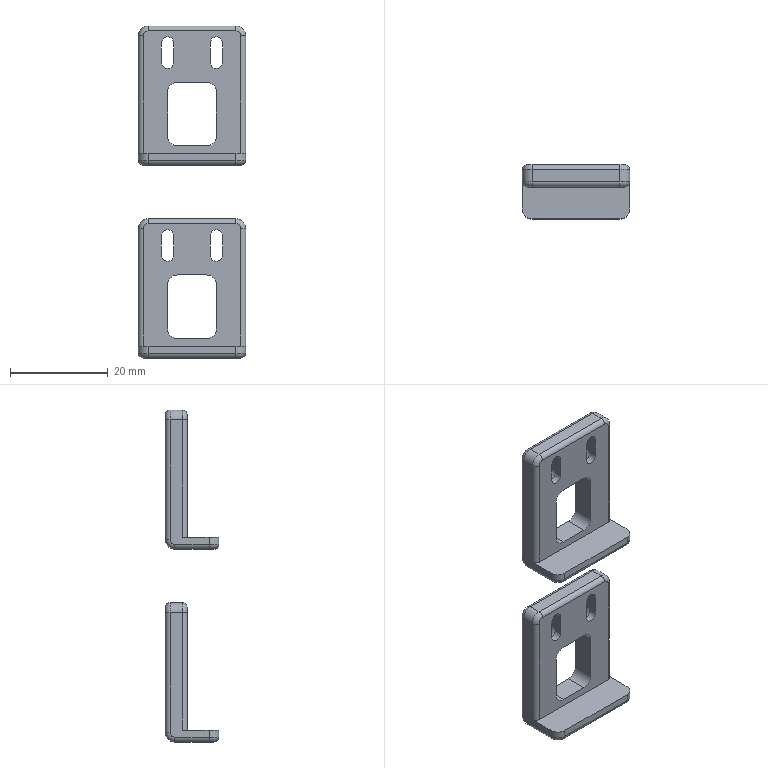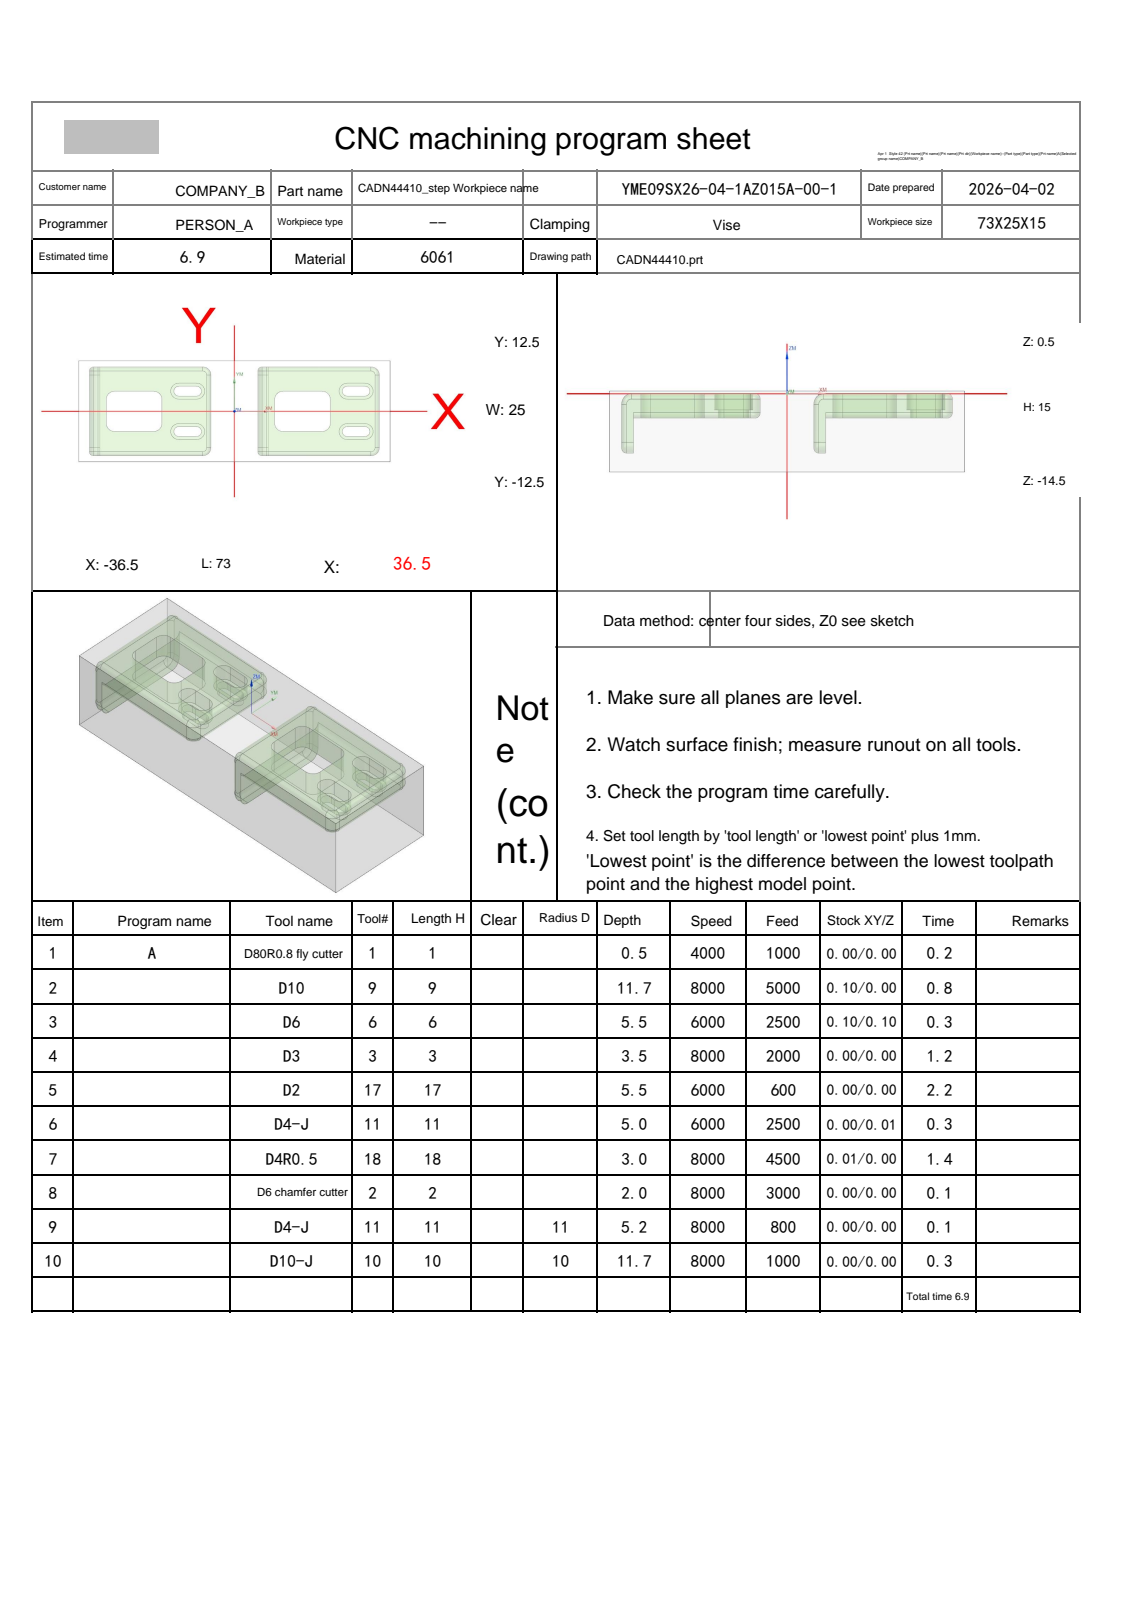NC program | NX | posted by the shop | part box 22 x 11 x 68 mm
Lines 1 to 969 of 7842:
%
O0001
(Machine time: 8.83 MIN)
(===Total Tool:9===)
(T1=D80R0.8 fly cutter D=80.  R=0.8 H01 Z=0.    )
(T9=D10     D=10.  R=0.   D-  H09 Z=-11.2 )
(T6=D6      D=6.   R=0.   D-  H06 Z=-5.   )
(T3=D3      D=3.   R=0.   D3  H03 Z=-3.   )
(T17=D2     D=2.   R=0.   D17 H17 Z=-5.   )
(T11=D4-J   D=4.   R=0.   D-  H11 Z=-4.7  )
(T18=D4R0.5 D=4.   R=0.5  D-  H18 Z=-2.5  )
(T2=D6 chamfer cutter   D=6.   R=0.   D-  H02 Z=-1.5  )
(T10=D10-J  D=10.  R=0.   D10 H10 Z=-11.2 )
G80 G90 G17 G49 G40
G91 G28 Z0
M01
N1 T01 M06
(D80R0.8 fly cutter D=80. R=0.8 H=01 ce=0.00 di=0.00)
G00 G90 G54 X79. Y0.0 M03 S4000
G43 H01 Z20.
M08
Z2.
G01 Z0.0 F1000.
X74.
X-74.
X-79.
Z2.
G00 Z20.
G91 G28 Z0.0
M05
M09
G91 G28 Z0.0
M01
N2 T09 M06
(D10  D=10. R=0. H=09 ce=0.10 di=0.00)
G00 G90 G54 X39.1 Y0.0 M03 S8000
G43 H09 Z20.
M08
Z.5
G01 Y-9.23 Z.445 F5000.
X39.009 Y-10.242 Z.439
X38.687 Y-11.449 Z.431
X38.147 Y-12.592 Z.424
X37.426 Y-13.609 Z.416
X36.542 Y-14.481 Z.409
X35.533 Y-15.18 Z.402
X34.408 Y-15.701 Z.394
X33.22 Y-16.012 Z.387
X32.226 Y-16.1 Z.381
X6.5 Z.227
G02 X.4 Y-10. Z.17 I0.0 J6.1
G01 Y10. Z.05
G02 X6.5 Y16.1 Z-.007 I6.1 J0.0
G01 X32.231 Z-.161
X33.243 Y16.008 Z-.167
X34.45 Y15.687 Z-.174
X35.593 Y15.146 Z-.182
X36.608 Y14.425 Z-.189
X37.478 Y13.544 Z-.197
X38.179 Y12.535 Z-.204
X38.702 Y11.406 Z-.212
X39.011 Y10.22 Z-.219
X39.1 Y9.228 Z-.225
Y-9.23 Z-.335
X39.009 Y-10.242 Z-.341
X38.687 Y-11.449 Z-.349
X38.147 Y-12.592 Z-.356
X37.426 Y-13.609 Z-.364
X36.542 Y-14.481 Z-.371
X35.533 Y-15.18 Z-.378
X34.408 Y-15.701 Z-.386
X33.22 Y-16.012 Z-.393
X32.226 Y-16.1 Z-.399
X6.5 Z-.553
G02 X.4 Y-10. Z-.61 I0.0 J6.1
G01 Y10. Z-.73
G02 X6.5 Y16.1 Z-.787 I6.1 J0.0
G01 X32.231 Z-.941
X33.243 Y16.008 Z-.947
X34.45 Y15.687 Z-.954
X35.593 Y15.146 Z-.962
X36.608 Y14.425 Z-.969
X37.478 Y13.544 Z-.977
X38.179 Y12.535 Z-.984
X38.702 Y11.406 Z-.992
X39.011 Y10.22 Z-.999
X39.1 Y9.228 Z-1.005
Y-9.23 Z-1.115
X39.009 Y-10.242 Z-1.121
X38.687 Y-11.449 Z-1.129
X38.147 Y-12.592 Z-1.136
X37.426 Y-13.609 Z-1.144
X36.542 Y-14.481 Z-1.151
X35.533 Y-15.18 Z-1.158
X34.408 Y-15.701 Z-1.166
X33.22 Y-16.012 Z-1.173
X32.226 Y-16.1 Z-1.179
X6.5 Z-1.333
G02 X.4 Y-10. Z-1.39 I0.0 J6.1
G01 Y10. Z-1.51
G02 X6.5 Y16.1 Z-1.567 I6.1 J0.0
G01 X32.231 Z-1.721
X33.243 Y16.008 Z-1.727
X34.45 Y15.687 Z-1.734
X35.593 Y15.146 Z-1.742
X36.608 Y14.425 Z-1.749
X37.478 Y13.544 Z-1.757
X38.179 Y12.535 Z-1.764
X38.702 Y11.406 Z-1.772
X39.011 Y10.22 Z-1.779
X39.1 Y9.228 Z-1.785
Y-9.23 Z-1.895
X39.009 Y-10.242 Z-1.901
X38.687 Y-11.449 Z-1.909
X38.147 Y-12.592 Z-1.916
X37.426 Y-13.609 Z-1.924
X36.542 Y-14.481 Z-1.931
X35.533 Y-15.18 Z-1.938
X34.408 Y-15.701 Z-1.946
X33.22 Y-16.012 Z-1.953
X32.226 Y-16.1 Z-1.959
X6.5 Z-2.113
G02 X.4 Y-10. Z-2.17 I0.0 J6.1
G01 Y10. Z-2.29
G02 X6.5 Y16.1 Z-2.347 I6.1 J0.0
G01 X32.231 Z-2.501
X33.243 Y16.008 Z-2.507
X34.45 Y15.687 Z-2.514
X35.593 Y15.146 Z-2.522
X36.608 Y14.425 Z-2.529
X37.478 Y13.544 Z-2.537
X38.179 Y12.535 Z-2.544
X38.702 Y11.406 Z-2.552
X39.011 Y10.22 Z-2.559
X39.1 Y9.228 Z-2.565
Y-9.23 Z-2.675
X39.009 Y-10.242 Z-2.681
X38.687 Y-11.449 Z-2.689
X38.147 Y-12.592 Z-2.696
X37.426 Y-13.609 Z-2.704
X36.542 Y-14.481 Z-2.711
X35.533 Y-15.18 Z-2.718
X34.408 Y-15.701 Z-2.726
X33.22 Y-16.012 Z-2.733
X32.226 Y-16.1 Z-2.739
X6.5 Z-2.893
G02 X.4 Y-10. Z-2.95 I0.0 J6.1
G01 Y10. Z-3.07
G02 X6.5 Y16.1 Z-3.127 I6.1 J0.0
G01 X32.231 Z-3.281
X33.243 Y16.008 Z-3.287
X34.45 Y15.687 Z-3.294
X35.593 Y15.146 Z-3.302
X36.608 Y14.425 Z-3.309
X37.478 Y13.544 Z-3.317
X38.179 Y12.535 Z-3.324
X38.702 Y11.406 Z-3.332
X39.011 Y10.22 Z-3.339
X39.1 Y9.228 Z-3.345
Y-9.23 Z-3.455
X39.009 Y-10.242 Z-3.461
X38.687 Y-11.449 Z-3.469
X38.147 Y-12.592 Z-3.476
X37.426 Y-13.609 Z-3.484
X36.542 Y-14.481 Z-3.491
X35.533 Y-15.18 Z-3.498
X34.408 Y-15.701 Z-3.506
X33.22 Y-16.012 Z-3.513
X32.226 Y-16.1 Z-3.519
X6.5 Z-3.673
G02 X.4 Y-10. Z-3.73 I0.0 J6.1
G01 Y10. Z-3.85
G02 X6.5 Y16.1 Z-3.907 I6.1 J0.0
G01 X32.231 Z-4.061
X33.243 Y16.008 Z-4.067
X34.45 Y15.687 Z-4.074
X35.593 Y15.146 Z-4.082
X36.608 Y14.425 Z-4.089
X37.478 Y13.544 Z-4.097
X38.179 Y12.535 Z-4.104
X38.702 Y11.406 Z-4.112
X39.011 Y10.22 Z-4.119
X39.1 Y9.228 Z-4.125
Y-9.23 Z-4.235
X39.009 Y-10.242 Z-4.241
X38.687 Y-11.449 Z-4.249
X38.147 Y-12.592 Z-4.256
X37.426 Y-13.609 Z-4.264
X36.542 Y-14.481 Z-4.271
X35.533 Y-15.18 Z-4.278
X34.408 Y-15.701 Z-4.286
X33.22 Y-16.012 Z-4.293
X32.226 Y-16.1 Z-4.299
X6.5 Z-4.453
G02 X.4 Y-10. Z-4.51 I0.0 J6.1
G01 Y10. Z-4.63
G02 X6.5 Y16.1 Z-4.687 I6.1 J0.0
G01 X32.231 Z-4.841
X33.243 Y16.008 Z-4.847
X34.45 Y15.687 Z-4.854
X35.593 Y15.146 Z-4.862
X36.608 Y14.425 Z-4.869
X37.478 Y13.544 Z-4.877
X38.179 Y12.535 Z-4.884
X38.702 Y11.406 Z-4.892
X39.011 Y10.22 Z-4.899
X39.1 Y9.228 Z-4.905
Y-9.23 Z-5.015
X39.009 Y-10.242 Z-5.021
X38.687 Y-11.449 Z-5.029
X38.147 Y-12.592 Z-5.036
X37.426 Y-13.609 Z-5.044
X36.542 Y-14.481 Z-5.051
X35.533 Y-15.18 Z-5.058
X34.408 Y-15.701 Z-5.066
X33.22 Y-16.012 Z-5.073
X32.226 Y-16.1 Z-5.079
X6.5 Z-5.233
G02 X.4 Y-10. Z-5.29 I0.0 J6.1
G01 Y10. Z-5.41
G02 X6.5 Y16.1 Z-5.467 I6.1 J0.0
G01 X32.231 Z-5.621
X33.243 Y16.008 Z-5.627
X34.45 Y15.687 Z-5.634
X35.593 Y15.146 Z-5.642
X36.608 Y14.425 Z-5.649
X37.478 Y13.544 Z-5.657
X38.179 Y12.535 Z-5.664
X38.702 Y11.406 Z-5.672
X39.011 Y10.22 Z-5.679
X39.1 Y9.228 Z-5.685
Y-9.23 Z-5.795
X39.009 Y-10.242 Z-5.801
X38.687 Y-11.449 Z-5.809
X38.147 Y-12.592 Z-5.816
X37.426 Y-13.609 Z-5.824
X36.542 Y-14.481 Z-5.831
X35.533 Y-15.18 Z-5.838
X34.408 Y-15.701 Z-5.846
X33.22 Y-16.012 Z-5.853
X32.226 Y-16.1 Z-5.859
X6.5 Z-6.013
G02 X.4 Y-10. Z-6.07 I0.0 J6.1
G01 Y10. Z-6.19
G02 X6.5 Y16.1 Z-6.247 I6.1 J0.0
G01 X32.231 Z-6.401
X33.243 Y16.008 Z-6.407
X34.45 Y15.687 Z-6.414
X35.593 Y15.146 Z-6.422
X36.608 Y14.425 Z-6.429
X37.478 Y13.544 Z-6.437
X38.179 Y12.535 Z-6.444
X38.702 Y11.406 Z-6.452
X39.011 Y10.22 Z-6.459
X39.1 Y9.228 Z-6.465
Y-9.23 Z-6.575
X39.009 Y-10.242 Z-6.581
X38.687 Y-11.449 Z-6.589
X38.147 Y-12.592 Z-6.596
X37.426 Y-13.609 Z-6.604
X36.542 Y-14.481 Z-6.611
X35.533 Y-15.18 Z-6.618
X34.408 Y-15.701 Z-6.626
X33.22 Y-16.012 Z-6.633
X32.226 Y-16.1 Z-6.639
X6.5 Z-6.793
G02 X.4 Y-10. Z-6.85 I0.0 J6.1
G01 Y10. Z-6.97
G02 X6.5 Y16.1 Z-7.027 I6.1 J0.0
G01 X32.231 Z-7.181
X33.243 Y16.008 Z-7.187
X34.45 Y15.687 Z-7.194
X35.593 Y15.146 Z-7.202
X36.608 Y14.425 Z-7.209
X37.478 Y13.544 Z-7.217
X38.179 Y12.535 Z-7.224
X38.702 Y11.406 Z-7.232
X39.011 Y10.22 Z-7.239
X39.1 Y9.228 Z-7.245
Y-9.23 Z-7.355
X39.009 Y-10.242 Z-7.361
X38.687 Y-11.449 Z-7.369
X38.147 Y-12.592 Z-7.376
X37.426 Y-13.609 Z-7.384
X36.542 Y-14.481 Z-7.391
X35.533 Y-15.18 Z-7.398
X34.408 Y-15.701 Z-7.406
X33.22 Y-16.012 Z-7.413
X32.226 Y-16.1 Z-7.419
X6.5 Z-7.573
G02 X.4 Y-10. Z-7.63 I0.0 J6.1
G01 Y10. Z-7.75
G02 X6.5 Y16.1 Z-7.807 I6.1 J0.0
G01 X32.231 Z-7.961
X33.243 Y16.008 Z-7.967
X34.45 Y15.687 Z-7.974
X35.593 Y15.146 Z-7.982
X36.608 Y14.425 Z-7.989
X37.478 Y13.544 Z-7.997
X38.179 Y12.535 Z-8.004
X38.702 Y11.406 Z-8.012
X39.011 Y10.22 Z-8.019
X39.1 Y9.228 Z-8.025
Y-9.23 Z-8.135
X39.009 Y-10.242 Z-8.141
X38.687 Y-11.449 Z-8.149
X38.147 Y-12.592 Z-8.156
X37.426 Y-13.609 Z-8.164
X36.542 Y-14.481 Z-8.171
X35.533 Y-15.18 Z-8.178
X34.408 Y-15.701 Z-8.186
X33.22 Y-16.012 Z-8.193
X32.226 Y-16.1 Z-8.199
X6.5 Z-8.353
G02 X.4 Y-10. Z-8.41 I0.0 J6.1
G01 Y10. Z-8.53
G02 X6.5 Y16.1 Z-8.587 I6.1 J0.0
G01 X32.231 Z-8.741
X33.243 Y16.008 Z-8.747
X34.45 Y15.687 Z-8.754
X35.593 Y15.146 Z-8.762
X36.608 Y14.425 Z-8.769
X37.478 Y13.544 Z-8.777
X38.179 Y12.535 Z-8.784
X38.702 Y11.406 Z-8.792
X39.011 Y10.22 Z-8.799
X39.1 Y9.228 Z-8.805
Y-9.23 Z-8.915
X39.009 Y-10.242 Z-8.921
X38.687 Y-11.449 Z-8.929
X38.147 Y-12.592 Z-8.936
X37.426 Y-13.609 Z-8.944
X36.542 Y-14.481 Z-8.951
X35.533 Y-15.18 Z-8.958
X34.408 Y-15.701 Z-8.966
X33.22 Y-16.012 Z-8.973
X32.226 Y-16.1 Z-8.979
X6.5 Z-9.133
G02 X.4 Y-10. Z-9.19 I0.0 J6.1
G01 Y10. Z-9.31
G02 X6.5 Y16.1 Z-9.367 I6.1 J0.0
G01 X32.231 Z-9.521
X33.243 Y16.008 Z-9.527
X34.45 Y15.687 Z-9.534
X35.593 Y15.146 Z-9.542
X36.608 Y14.425 Z-9.549
X37.478 Y13.544 Z-9.557
X38.179 Y12.535 Z-9.564
X38.702 Y11.406 Z-9.572
X39.011 Y10.22 Z-9.579
X39.1 Y9.228 Z-9.585
Y-9.23 Z-9.695
X39.009 Y-10.242 Z-9.701
X38.687 Y-11.449 Z-9.709
X38.147 Y-12.592 Z-9.716
X37.426 Y-13.609 Z-9.724
X36.542 Y-14.481 Z-9.731
X35.533 Y-15.18 Z-9.738
X34.408 Y-15.701 Z-9.746
X33.22 Y-16.012 Z-9.753
X32.226 Y-16.1 Z-9.759
X6.5 Z-9.913
G02 X.4 Y-10. Z-9.97 I0.0 J6.1
G01 Y10. Z-10.09
G02 X6.5 Y16.1 Z-10.147 I6.1 J0.0
G01 X32.231 Z-10.301
X33.243 Y16.008 Z-10.307
X34.45 Y15.687 Z-10.314
X35.593 Y15.146 Z-10.322
X36.608 Y14.425 Z-10.329
X37.478 Y13.544 Z-10.337
X38.179 Y12.535 Z-10.344
X38.702 Y11.406 Z-10.352
X39.011 Y10.22 Z-10.359
X39.1 Y9.228 Z-10.365
Y-9.23 Z-10.475
X39.009 Y-10.242 Z-10.481
X38.687 Y-11.449 Z-10.489
X38.147 Y-12.592 Z-10.496
X37.426 Y-13.609 Z-10.504
X36.542 Y-14.481 Z-10.511
X35.533 Y-15.18 Z-10.518
X34.408 Y-15.701 Z-10.526
X33.22 Y-16.012 Z-10.533
X32.226 Y-16.1 Z-10.539
X6.5 Z-10.693
G02 X.4 Y-10. Z-10.75 I0.0 J6.1
G01 Y10. Z-10.87
G02 X6.5 Y16.1 Z-10.927 I6.1 J0.0
G01 X32.231 Z-11.081
X33.243 Y16.008 Z-11.087
X34.45 Y15.687 Z-11.094
X35.593 Y15.146 Z-11.102
X36.608 Y14.425 Z-11.109
X37.478 Y13.544 Z-11.117
X38.179 Y12.535 Z-11.124
X38.702 Y11.406 Z-11.132
X39.011 Y10.22 Z-11.139
X39.1 Y9.228 Z-11.145
Y0.0 Z-11.2
Y-9.23
X39.009 Y-10.242
X38.687 Y-11.449
X38.147 Y-12.592
X37.426 Y-13.609
X36.542 Y-14.481
X35.533 Y-15.18
X34.408 Y-15.701
X33.22 Y-16.012
X32.226 Y-16.1
X6.5
G02 X.4 Y-10. I0.0 J6.1
G01 Y10.
G02 X6.5 Y16.1 I6.1 J0.0
G01 X32.231
X33.243 Y16.008
X34.45 Y15.687
X35.593 Y15.146
X36.608 Y14.425
X37.478 Y13.544
X38.179 Y12.535
X38.702 Y11.406
X39.011 Y10.22
X39.1 Y9.228
Y0.0
Y-.5
Z-10.2
G00 Z20.
X-.4 Y0.0
Z.5
G01 Y-9.23 Z.445
X-.491 Y-10.242 Z.439
X-.813 Y-11.449 Z.431
X-1.353 Y-12.592 Z.424
X-2.074 Y-13.609 Z.416
X-2.958 Y-14.481 Z.409
X-3.967 Y-15.18 Z.402
X-5.092 Y-15.701 Z.394
X-6.28 Y-16.012 Z.387
X-7.274 Y-16.1 Z.381
X-33. Z.227
G02 X-39.1 Y-10. Z.17 I0.0 J6.1
G01 Y10. Z.05
G02 X-33. Y16.1 Z-.007 I6.1 J0.0
G01 X-7.269 Z-.161
X-6.257 Y16.008 Z-.167
X-5.05 Y15.687 Z-.174
X-3.907 Y15.146 Z-.182
X-2.892 Y14.425 Z-.189
X-2.022 Y13.544 Z-.197
X-1.321 Y12.535 Z-.204
X-.798 Y11.406 Z-.212
X-.489 Y10.22 Z-.219
X-.4 Y9.228 Z-.225
Y-9.23 Z-.335
X-.491 Y-10.242 Z-.341
X-.813 Y-11.449 Z-.349
X-1.353 Y-12.592 Z-.356
X-2.074 Y-13.609 Z-.364
X-2.958 Y-14.481 Z-.371
X-3.967 Y-15.18 Z-.378
X-5.092 Y-15.701 Z-.386
X-6.28 Y-16.012 Z-.393
X-7.274 Y-16.1 Z-.399
X-33. Z-.553
G02 X-39.1 Y-10. Z-.61 I0.0 J6.1
G01 Y10. Z-.73
G02 X-33. Y16.1 Z-.787 I6.1 J0.0
G01 X-7.269 Z-.941
X-6.257 Y16.008 Z-.947
X-5.05 Y15.687 Z-.954
X-3.907 Y15.146 Z-.962
X-2.892 Y14.425 Z-.969
X-2.022 Y13.544 Z-.977
X-1.321 Y12.535 Z-.984
X-.798 Y11.406 Z-.992
X-.489 Y10.22 Z-.999
X-.4 Y9.228 Z-1.005
Y-9.23 Z-1.115
X-.491 Y-10.242 Z-1.121
X-.813 Y-11.449 Z-1.129
X-1.353 Y-12.592 Z-1.136
X-2.074 Y-13.609 Z-1.144
X-2.958 Y-14.481 Z-1.151
X-3.967 Y-15.18 Z-1.158
X-5.092 Y-15.701 Z-1.166
X-6.28 Y-16.012 Z-1.173
X-7.274 Y-16.1 Z-1.179
X-33. Z-1.333
G02 X-39.1 Y-10. Z-1.39 I0.0 J6.1
G01 Y10. Z-1.51
G02 X-33. Y16.1 Z-1.567 I6.1 J0.0
G01 X-7.269 Z-1.721
X-6.257 Y16.008 Z-1.727
X-5.05 Y15.687 Z-1.734
X-3.907 Y15.146 Z-1.742
X-2.892 Y14.425 Z-1.749
X-2.022 Y13.544 Z-1.757
X-1.321 Y12.535 Z-1.764
X-.798 Y11.406 Z-1.772
X-.489 Y10.22 Z-1.779
X-.4 Y9.228 Z-1.785
Y-9.23 Z-1.895
X-.491 Y-10.242 Z-1.901
X-.813 Y-11.449 Z-1.909
X-1.353 Y-12.592 Z-1.916
X-2.074 Y-13.609 Z-1.924
X-2.958 Y-14.481 Z-1.931
X-3.967 Y-15.18 Z-1.938
X-5.092 Y-15.701 Z-1.946
X-6.28 Y-16.012 Z-1.953
X-7.274 Y-16.1 Z-1.959
X-33. Z-2.113
G02 X-39.1 Y-10. Z-2.17 I0.0 J6.1
G01 Y10. Z-2.29
G02 X-33. Y16.1 Z-2.347 I6.1 J0.0
G01 X-7.269 Z-2.501
X-6.257 Y16.008 Z-2.507
X-5.05 Y15.687 Z-2.514
X-3.907 Y15.146 Z-2.522
X-2.892 Y14.425 Z-2.529
X-2.022 Y13.544 Z-2.537
X-1.321 Y12.535 Z-2.544
X-.798 Y11.406 Z-2.552
X-.489 Y10.22 Z-2.559
X-.4 Y9.228 Z-2.565
Y-9.23 Z-2.675
X-.491 Y-10.242 Z-2.681
X-.813 Y-11.449 Z-2.689
X-1.353 Y-12.592 Z-2.696
X-2.074 Y-13.609 Z-2.704
X-2.958 Y-14.481 Z-2.711
X-3.967 Y-15.18 Z-2.718
X-5.092 Y-15.701 Z-2.726
X-6.28 Y-16.012 Z-2.733
X-7.274 Y-16.1 Z-2.739
X-33. Z-2.893
G02 X-39.1 Y-10. Z-2.95 I0.0 J6.1
G01 Y10. Z-3.07
G02 X-33. Y16.1 Z-3.127 I6.1 J0.0
G01 X-7.269 Z-3.281
X-6.257 Y16.008 Z-3.287
X-5.05 Y15.687 Z-3.294
X-3.907 Y15.146 Z-3.302
X-2.892 Y14.425 Z-3.309
X-2.022 Y13.544 Z-3.317
X-1.321 Y12.535 Z-3.324
X-.798 Y11.406 Z-3.332
X-.489 Y10.22 Z-3.339
X-.4 Y9.228 Z-3.345
Y-9.23 Z-3.455
X-.491 Y-10.242 Z-3.461
X-.813 Y-11.449 Z-3.469
X-1.353 Y-12.592 Z-3.476
X-2.074 Y-13.609 Z-3.484
X-2.958 Y-14.481 Z-3.491
X-3.967 Y-15.18 Z-3.498
X-5.092 Y-15.701 Z-3.506
X-6.28 Y-16.012 Z-3.513
X-7.274 Y-16.1 Z-3.519
X-33. Z-3.673
G02 X-39.1 Y-10. Z-3.73 I0.0 J6.1
G01 Y10. Z-3.85
G02 X-33. Y16.1 Z-3.907 I6.1 J0.0
G01 X-7.269 Z-4.061
X-6.257 Y16.008 Z-4.067
X-5.05 Y15.687 Z-4.074
X-3.907 Y15.146 Z-4.082
X-2.892 Y14.425 Z-4.089
X-2.022 Y13.544 Z-4.097
X-1.321 Y12.535 Z-4.104
X-.798 Y11.406 Z-4.112
X-.489 Y10.22 Z-4.119
X-.4 Y9.228 Z-4.125
Y-9.23 Z-4.235
X-.491 Y-10.242 Z-4.241
X-.813 Y-11.449 Z-4.249
X-1.353 Y-12.592 Z-4.256
X-2.074 Y-13.609 Z-4.264
X-2.958 Y-14.481 Z-4.271
X-3.967 Y-15.18 Z-4.278
X-5.092 Y-15.701 Z-4.286
X-6.28 Y-16.012 Z-4.293
X-7.274 Y-16.1 Z-4.299
X-33. Z-4.453
G02 X-39.1 Y-10. Z-4.51 I0.0 J6.1
G01 Y10. Z-4.63
G02 X-33. Y16.1 Z-4.687 I6.1 J0.0
G01 X-7.269 Z-4.841
X-6.257 Y16.008 Z-4.847
X-5.05 Y15.687 Z-4.854
X-3.907 Y15.146 Z-4.862
X-2.892 Y14.425 Z-4.869
X-2.022 Y13.544 Z-4.877
X-1.321 Y12.535 Z-4.884
X-.798 Y11.406 Z-4.892
X-.489 Y10.22 Z-4.899
X-.4 Y9.228 Z-4.905
Y-9.23 Z-5.015
X-.491 Y-10.242 Z-5.021
X-.813 Y-11.449 Z-5.029
X-1.353 Y-12.592 Z-5.036
X-2.074 Y-13.609 Z-5.044
X-2.958 Y-14.481 Z-5.051
X-3.967 Y-15.18 Z-5.058
X-5.092 Y-15.701 Z-5.066
X-6.28 Y-16.012 Z-5.073
X-7.274 Y-16.1 Z-5.079
X-33. Z-5.233
G02 X-39.1 Y-10. Z-5.29 I0.0 J6.1
G01 Y10. Z-5.41
G02 X-33. Y16.1 Z-5.467 I6.1 J0.0
G01 X-7.269 Z-5.621
X-6.257 Y16.008 Z-5.627
X-5.05 Y15.687 Z-5.634
X-3.907 Y15.146 Z-5.642
X-2.892 Y14.425 Z-5.649
X-2.022 Y13.544 Z-5.657
X-1.321 Y12.535 Z-5.664
X-.798 Y11.406 Z-5.672
X-.489 Y10.22 Z-5.679
X-.4 Y9.228 Z-5.685
Y-9.23 Z-5.795
X-.491 Y-10.242 Z-5.801
X-.813 Y-11.449 Z-5.809
X-1.353 Y-12.592 Z-5.816
X-2.074 Y-13.609 Z-5.824
X-2.958 Y-14.481 Z-5.831
X-3.967 Y-15.18 Z-5.838
X-5.092 Y-15.701 Z-5.846
X-6.28 Y-16.012 Z-5.853
X-7.274 Y-16.1 Z-5.859
X-33. Z-6.013
G02 X-39.1 Y-10. Z-6.07 I0.0 J6.1
G01 Y10. Z-6.19
G02 X-33. Y16.1 Z-6.247 I6.1 J0.0
G01 X-7.269 Z-6.401
X-6.257 Y16.008 Z-6.407
X-5.05 Y15.687 Z-6.414
X-3.907 Y15.146 Z-6.422
X-2.892 Y14.425 Z-6.429
X-2.022 Y13.544 Z-6.437
X-1.321 Y12.535 Z-6.444
X-.798 Y11.406 Z-6.452
X-.489 Y10.22 Z-6.459
X-.4 Y9.228 Z-6.465
Y-9.23 Z-6.575
X-.491 Y-10.242 Z-6.581
X-.813 Y-11.449 Z-6.589
X-1.353 Y-12.592 Z-6.596
X-2.074 Y-13.609 Z-6.604
X-2.958 Y-14.481 Z-6.611
X-3.967 Y-15.18 Z-6.618
X-5.092 Y-15.701 Z-6.626
X-6.28 Y-16.012 Z-6.633
X-7.274 Y-16.1 Z-6.639
X-33. Z-6.793
G02 X-39.1 Y-10. Z-6.85 I0.0 J6.1
G01 Y10. Z-6.97
G02 X-33. Y16.1 Z-7.027 I6.1 J0.0
G01 X-7.269 Z-7.181
X-6.257 Y16.008 Z-7.187
X-5.05 Y15.687 Z-7.194
X-3.907 Y15.146 Z-7.202
X-2.892 Y14.425 Z-7.209
X-2.022 Y13.544 Z-7.217
X-1.321 Y12.535 Z-7.224
X-.798 Y11.406 Z-7.232
X-.489 Y10.22 Z-7.239
X-.4 Y9.228 Z-7.245
Y-9.23 Z-7.355
X-.491 Y-10.242 Z-7.361
X-.813 Y-11.449 Z-7.369
X-1.353 Y-12.592 Z-7.376
X-2.074 Y-13.609 Z-7.384
X-2.958 Y-14.481 Z-7.391
X-3.967 Y-15.18 Z-7.398
X-5.092 Y-15.701 Z-7.406
X-6.28 Y-16.012 Z-7.413
X-7.274 Y-16.1 Z-7.419
X-33. Z-7.573
G02 X-39.1 Y-10. Z-7.63 I0.0 J6.1
G01 Y10. Z-7.75
G02 X-33. Y16.1 Z-7.807 I6.1 J0.0
G01 X-7.269 Z-7.961
X-6.257 Y16.008 Z-7.967
X-5.05 Y15.687 Z-7.974
X-3.907 Y15.146 Z-7.982
X-2.892 Y14.425 Z-7.989
X-2.022 Y13.544 Z-7.997
X-1.321 Y12.535 Z-8.004
X-.798 Y11.406 Z-8.012
X-.489 Y10.22 Z-8.019
X-.4 Y9.228 Z-8.025
Y-9.23 Z-8.135
X-.491 Y-10.242 Z-8.141
X-.813 Y-11.449 Z-8.149
X-1.353 Y-12.592 Z-8.156
X-2.074 Y-13.609 Z-8.164
X-2.958 Y-14.481 Z-8.171
X-3.967 Y-15.18 Z-8.178
X-5.092 Y-15.701 Z-8.186
X-6.28 Y-16.012 Z-8.193
X-7.274 Y-16.1 Z-8.199
X-33. Z-8.353
G02 X-39.1 Y-10. Z-8.41 I0.0 J6.1
G01 Y10. Z-8.53
G02 X-33. Y16.1 Z-8.587 I6.1 J0.0
G01 X-7.269 Z-8.741
X-6.257 Y16.008 Z-8.747
X-5.05 Y15.687 Z-8.754
X-3.907 Y15.146 Z-8.762
X-2.892 Y14.425 Z-8.769
X-2.022 Y13.544 Z-8.777
X-1.321 Y12.535 Z-8.784
X-.798 Y11.406 Z-8.792
X-.489 Y10.22 Z-8.799
X-.4 Y9.228 Z-8.805
Y-9.23 Z-8.915
X-.491 Y-10.242 Z-8.921
X-.813 Y-11.449 Z-8.929
X-1.353 Y-12.592 Z-8.936
X-2.074 Y-13.609 Z-8.944
X-2.958 Y-14.481 Z-8.951
X-3.967 Y-15.18 Z-8.958
X-5.092 Y-15.701 Z-8.966
X-6.28 Y-16.012 Z-8.973
X-7.274 Y-16.1 Z-8.979
X-33. Z-9.133
G02 X-39.1 Y-10. Z-9.19 I0.0 J6.1
G01 Y10. Z-9.31
G02 X-33. Y16.1 Z-9.367 I6.1 J0.0
G01 X-7.269 Z-9.521
X-6.257 Y16.008 Z-9.527
X-5.05 Y15.687 Z-9.534
X-3.907 Y15.146 Z-9.542
X-2.892 Y14.425 Z-9.549
X-2.022 Y13.544 Z-9.557
X-1.321 Y12.535 Z-9.564
X-.798 Y11.406 Z-9.572
X-.489 Y10.22 Z-9.579
X-.4 Y9.228 Z-9.585
Y-9.23 Z-9.695
X-.491 Y-10.242 Z-9.701
X-.813 Y-11.449 Z-9.709
X-1.353 Y-12.592 Z-9.716
X-2.074 Y-13.609 Z-9.724
X-2.958 Y-14.481 Z-9.731
X-3.967 Y-15.18 Z-9.738
X-5.092 Y-15.701 Z-9.746
X-6.28 Y-16.012 Z-9.753
X-7.274 Y-16.1 Z-9.759
X-33. Z-9.913
G02 X-39.1 Y-10. Z-9.97 I0.0 J6.1
G01 Y10. Z-10.09
G02 X-33. Y16.1 Z-10.147 I6.1 J0.0
G01 X-7.269 Z-10.301
X-6.257 Y16.008 Z-10.307
X-5.05 Y15.687 Z-10.314
X-3.907 Y15.146 Z-10.322
X-2.892 Y14.425 Z-10.329
X-2.022 Y13.544 Z-10.337
X-1.321 Y12.535 Z-10.344
X-.798 Y11.406 Z-10.352
X-.489 Y10.22 Z-10.359
X-.4 Y9.228 Z-10.365
Y-9.23 Z-10.475
X-.491 Y-10.242 Z-10.481
X-.813 Y-11.449 Z-10.489
X-1.353 Y-12.592 Z-10.496
X-2.074 Y-13.609 Z-10.504
X-2.958 Y-14.481 Z-10.511
X-3.967 Y-15.18 Z-10.518
X-5.092 Y-15.701 Z-10.526
X-6.28 Y-16.012 Z-10.533
X-7.274 Y-16.1 Z-10.539
X-33. Z-10.693
G02 X-39.1 Y-10. Z-10.75 I0.0 J6.1
G01 Y10. Z-10.87
G02 X-33. Y16.1 Z-10.927 I6.1 J0.0
G01 X-7.269 Z-11.081
X-6.257 Y16.008 Z-11.087
X-5.05 Y15.687 Z-11.094
X-3.907 Y15.146 Z-11.102
X-2.892 Y14.425 Z-11.109
X-2.022 Y13.544 Z-11.117
X-1.321 Y12.535 Z-11.124
X-.798 Y11.406 Z-11.132
X-.489 Y10.22 Z-11.139
X-.4 Y9.228 Z-11.145
Y0.0 Z-11.2
Y-9.23
X-.491 Y-10.242
X-.813 Y-11.449
X-1.353 Y-12.592
X-2.074 Y-13.609
X-2.958 Y-14.481
X-3.967 Y-15.18
X-5.092 Y-15.701
X-6.28 Y-16.012
X-7.274 Y-16.1
X-33.
G02 X-39.1 Y-10. I0.0 J6.1
G01 Y10.
G02 X-33. Y16.1 I6.1 J0.0
G01 X-7.269
X-6.257 Y16.008
X-5.05 Y15.687
X-3.907 Y15.146
X-2.892 Y14.425
X-2.022 Y13.544
X-1.321 Y12.535
X-.798 Y11.406
X-.489 Y10.22
X-.4 Y9.228
Y0.0
Y-.5
Z-10.2
G00 Z20.
G91 G28 Z0.0
M05
M09
G91 G28 Z0.0
M01
N3 T06 M06
(D6  D=6. R=0. H=06 ce=0.10 di=0.10)
G00 G90 G54 X15.975 Y1.9 M03 S6000
G43 H06 Z20.
M08
Z.5
G01 X12.55 Z.437 F2500.
Y-1.9 Z.367
X19.4 Z.24
Y1.9 Z.17
X12.55 Z.044
Y-1.9 Z-.026
X19.4 Z-.152
Y1.9 Z-.223
X12.55 Z-.349
Y-1.9 Z-.419
X19.4 Z-.545
Y1.9 Z-.615
X12.55 Z-.742
Y-1.9 Z-.812
X19.4 Z-.938
Y1.9 Z-1.008
X12.55 Z-1.135
Y-1.9 Z-1.205
X19.4 Z-1.331
Y1.9 Z-1.401
X12.55 Z-1.527
Y-1.9 Z-1.598
X19.4 Z-1.724
Y1.9 Z-1.794
X12.55 Z-1.92
Y-1.9 Z-1.99
X19.4 Z-2.117
Y1.9 Z-2.187
X12.55 Z-2.313
Y-1.9 Z-2.383
X19.4 Z-2.51
Y1.9 Z-2.58
X12.55 Z-2.706
Y-1.9 Z-2.776
X19.4 Z-2.902
Y1.9 Z-2.973
X12.55 Z-3.099
Y-1.9 Z-3.169
X19.4 Z-3.295
Y1.9 Z-3.365
X12.55 Z-3.492
Y-1.9 Z-3.562
X19.4 Z-3.688
Y1.9 Z-3.758
X12.55 Z-3.885
Y-1.9 Z-3.955
X19.4 Z-4.081
Y1.9 Z-4.151
X12.55 Z-4.277
Y-1.9 Z-4.348
X19.4 Z-4.474
Y1.9 Z-4.544
X12.55 Z-4.67
Y-1.9 Z-4.74
X19.4 Z-4.867
Y1.9 Z-4.937
X15.975 Z-5.
X12.55
Y-1.9
X19.4
Y1.9
X15.975
X15.475
Z-4.
G00 Z20.
X-23.525
Z.5
G01 X-26.95 Z.437
Y-1.9 Z.367
X-20.1 Z.24
Y1.9 Z.17
X-26.95 Z.044
Y-1.9 Z-.026
X-20.1 Z-.152
Y1.9 Z-.223
X-26.95 Z-.349
Y-1.9 Z-.419
X-20.1 Z-.545
Y1.9 Z-.615
X-26.95 Z-.742
Y-1.9 Z-.812
X-20.1 Z-.938
Y1.9 Z-1.008
X-26.95 Z-1.135
Y-1.9 Z-1.205
X-20.1 Z-1.331
Y1.9 Z-1.401
X-26.95 Z-1.527
Y-1.9 Z-1.598
X-20.1 Z-1.724
Y1.9 Z-1.794
X-26.95 Z-1.92
Y-1.9 Z-1.99
X-20.1 Z-2.117
Y1.9 Z-2.187
X-26.95 Z-2.313
Y-1.9 Z-2.383
X-20.1 Z-2.51
Y1.9 Z-2.58
X-26.95 Z-2.706
Y-1.9 Z-2.776
X-20.1 Z-2.902
Y1.9 Z-2.973
X-26.95 Z-3.099
Y-1.9 Z-3.169
X-20.1 Z-3.295
Y1.9 Z-3.365
X-26.95 Z-3.492
Y-1.9 Z-3.562
X-20.1 Z-3.688
Y1.9 Z-3.758
X-26.95 Z-3.885
Y-1.9 Z-3.955
X-20.1 Z-4.081
Y1.9 Z-4.151
X-26.95 Z-4.277
Y-1.9 Z-4.348
X-20.1 Z-4.474
Y1.9 Z-4.544
X-26.95 Z-4.67
Y-1.9 Z-4.74
X-20.1 Z-4.867
Y1.9 Z-4.937
X-23.525 Z-5.
X-26.95
Y-1.9
X-20.1
Y1.9
X-23.525
X-24.025
Z-4.
G00 Z20.
G91 G28 Z0.0
M05
M09
G91 G28 Z0.0
M01